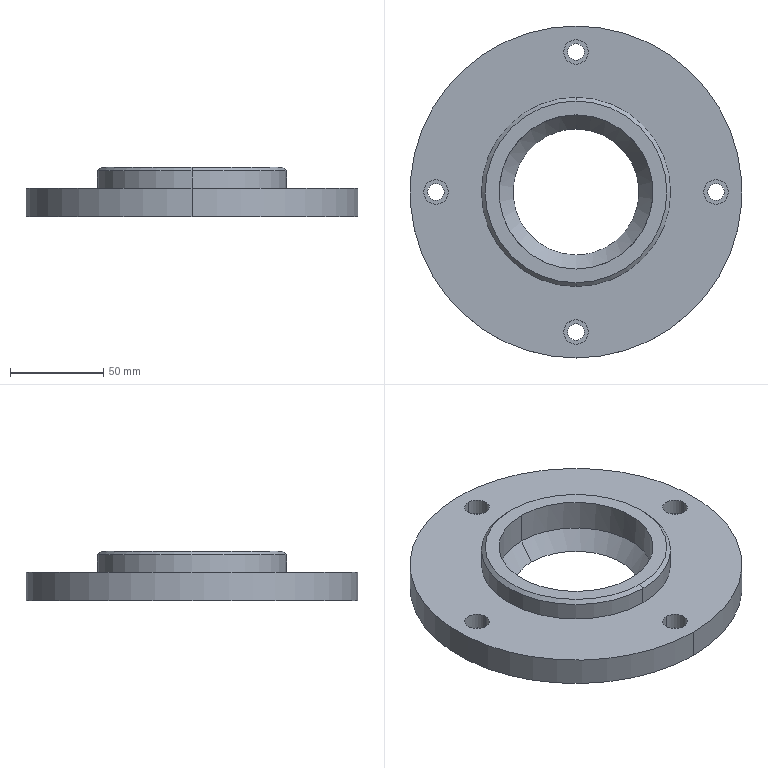Part | STEP file | 4-20.sldasm-Part-429 | 1 solid | 33 faces | box 177.8 x 177.8 x 26.75 mm | volume 331383 mm3 | cylinder 22 | plane 7 | spline 2 | cone 2 | commonest cylinder face diameters 8.931 x8 13.145 x8 82.56 x2 101.34 x2 177.8 x2
STEP:
#1=CARTESIAN_POINT('',(0.,81.572,313.382));
#2=VERTEX_POINT('',#1);
#3=CARTESIAN_POINT('',(0.,68.428,313.382));
#4=VERTEX_POINT('',#3);
#5=CARTESIAN_POINT('',(0.,75.,313.382));
#6=DIRECTION('',(0.,0.,1.));
#7=DIRECTION('',(0.,1.,0.));
#8=AXIS2_PLACEMENT_3D('',#5,#6,#7);
#9=CIRCLE('',#8,6.572);
#10=EDGE_CURVE('',#2,#4,#9,.T.);
#11=ORIENTED_EDGE('',*,*,#10,.F.);
#12=CARTESIAN_POINT('',(0.,81.572,322.275));
#13=VERTEX_POINT('',#12);
#14=CARTESIAN_POINT('',(0.,81.572,270.665));
#15=DIRECTION('',(0.,0.,1.));
#16=VECTOR('',#15,1000.);
#17=LINE('',#14,#16);
#18=EDGE_CURVE('',#2,#13,#17,.T.);
#19=ORIENTED_EDGE('',*,*,#18,.T.);
#20=CARTESIAN_POINT('',(0.,68.428,322.275));
#21=VERTEX_POINT('',#20);
#22=CARTESIAN_POINT('',(0.,75.,322.275));
#23=DIRECTION('',(0.,0.,-1.));
#24=DIRECTION('',(0.,-1.,0.));
#25=AXIS2_PLACEMENT_3D('',#22,#23,#24);
#26=CIRCLE('',#25,6.572);
#27=EDGE_CURVE('',#21,#13,#26,.T.);
#28=ORIENTED_EDGE('',*,*,#27,.F.);
#29=CARTESIAN_POINT('',(0.,68.428,270.665));
#30=DIRECTION('',(0.,0.,1.));
#31=VECTOR('',#30,1000.);
#32=LINE('',#29,#31);
#33=EDGE_CURVE('',#4,#21,#32,.T.);
#34=ORIENTED_EDGE('',*,*,#33,.F.);
#35=EDGE_LOOP('',(#11,#19,#28,#34));
#36=FACE_OUTER_BOUND('',#35,.T.);
#37=CARTESIAN_POINT('',(0.,75.,270.665));
#38=DIRECTION('',(0.,0.,1.));
#39=DIRECTION('',(0.,-1.,0.));
#40=AXIS2_PLACEMENT_3D('',#37,#38,#39);
#41=CYLINDRICAL_SURFACE('',#40,6.572);
#42=ADVANCED_FACE('',(#36),#41,.F.);
#43=CARTESIAN_POINT('',(-4.465,75.,313.382));
#44=VERTEX_POINT('',#43);
#45=CARTESIAN_POINT('',(4.465,75.,313.382));
#46=VERTEX_POINT('',#45);
#47=CARTESIAN_POINT('',(0.,75.,313.382));
#48=DIRECTION('',(0.,0.,-1.));
#49=DIRECTION('',(1.,0.,0.));
#50=AXIS2_PLACEMENT_3D('',#47,#48,#49);
#51=CIRCLE('',#50,4.465);
#52=EDGE_CURVE('',#44,#46,#51,.T.);
#53=ORIENTED_EDGE('',*,*,#52,.F.);
#54=CARTESIAN_POINT('',(-4.465,75.,306.955));
#55=VERTEX_POINT('',#54);
#56=CARTESIAN_POINT('',(-4.465,75.,313.382));
#57=DIRECTION('',(0.,0.,-1.));
#58=VECTOR('',#57,1000.);
#59=LINE('',#56,#58);
#60=EDGE_CURVE('',#44,#55,#59,.T.);
#61=ORIENTED_EDGE('',*,*,#60,.T.);
#62=CARTESIAN_POINT('',(4.465,75.,306.955));
#63=VERTEX_POINT('',#62);
#64=CARTESIAN_POINT('',(0.,75.,306.955));
#65=DIRECTION('',(0.,-0.000000019,1.));
#66=DIRECTION('',(0.,-1.,-0.000000019));
#67=AXIS2_PLACEMENT_3D('',#64,#65,#66);
#68=CIRCLE('',#67,4.465);
#69=EDGE_CURVE('',#63,#55,#68,.T.);
#70=ORIENTED_EDGE('',*,*,#69,.F.);
#71=CARTESIAN_POINT('',(4.465,75.,313.382));
#72=DIRECTION('',(0.,0.,-1.));
#73=VECTOR('',#72,1000.);
#74=LINE('',#71,#73);
#75=EDGE_CURVE('',#46,#63,#74,.T.);
#76=ORIENTED_EDGE('',*,*,#75,.F.);
#77=EDGE_LOOP('',(#53,#61,#70,#76));
#78=FACE_OUTER_BOUND('',#77,.T.);
#79=CARTESIAN_POINT('',(0.,75.,313.382));
#80=DIRECTION('',(0.,0.,-1.));
#81=DIRECTION('',(1.,0.,0.));
#82=AXIS2_PLACEMENT_3D('',#79,#80,#81);
#83=CYLINDRICAL_SURFACE('',#82,4.465);
#84=ADVANCED_FACE('',(#78),#83,.F.);
#85=CARTESIAN_POINT('',(81.572,0.,313.382));
#86=VERTEX_POINT('',#85);
#87=CARTESIAN_POINT('',(68.428,0.,313.382));
#88=VERTEX_POINT('',#87);
#89=CARTESIAN_POINT('',(75.,0.,313.382));
#90=DIRECTION('',(0.,0.,1.));
#91=DIRECTION('',(1.,0.,0.));
#92=AXIS2_PLACEMENT_3D('',#89,#90,#91);
#93=CIRCLE('',#92,6.572);
#94=EDGE_CURVE('',#86,#88,#93,.T.);
#95=ORIENTED_EDGE('',*,*,#94,.F.);
#96=CARTESIAN_POINT('',(81.572,0.,322.275));
#97=VERTEX_POINT('',#96);
#98=CARTESIAN_POINT('',(81.572,0.,270.665));
#99=DIRECTION('',(0.,0.,1.));
#100=VECTOR('',#99,1000.);
#101=LINE('',#98,#100);
#102=EDGE_CURVE('',#86,#97,#101,.T.);
#103=ORIENTED_EDGE('',*,*,#102,.T.);
#104=CARTESIAN_POINT('',(68.428,0.,322.275));
#105=VERTEX_POINT('',#104);
#106=CARTESIAN_POINT('',(75.,0.,322.275));
#107=DIRECTION('',(0.,0.,-1.));
#108=DIRECTION('',(-1.,0.,0.));
#109=AXIS2_PLACEMENT_3D('',#106,#107,#108);
#110=CIRCLE('',#109,6.572);
#111=EDGE_CURVE('',#105,#97,#110,.T.);
#112=ORIENTED_EDGE('',*,*,#111,.F.);
#113=CARTESIAN_POINT('',(68.428,0.,270.665));
#114=DIRECTION('',(0.,0.,1.));
#115=VECTOR('',#114,1000.);
#116=LINE('',#113,#115);
#117=EDGE_CURVE('',#88,#105,#116,.T.);
#118=ORIENTED_EDGE('',*,*,#117,.F.);
#119=EDGE_LOOP('',(#95,#103,#112,#118));
#120=FACE_OUTER_BOUND('',#119,.T.);
#121=CARTESIAN_POINT('',(75.,0.,270.665));
#122=DIRECTION('',(0.,0.,1.));
#123=DIRECTION('',(-1.,0.,0.));
#124=AXIS2_PLACEMENT_3D('',#121,#122,#123);
#125=CYLINDRICAL_SURFACE('',#124,6.572);
#126=ADVANCED_FACE('',(#120),#125,.F.);
#127=CARTESIAN_POINT('',(75.,4.465,313.382));
#128=VERTEX_POINT('',#127);
#129=CARTESIAN_POINT('',(75.,-4.465,313.382));
#130=VERTEX_POINT('',#129);
#131=CARTESIAN_POINT('',(75.,0.,313.382));
#132=DIRECTION('',(0.,0.,-1.));
#133=DIRECTION('',(0.,-1.,0.));
#134=AXIS2_PLACEMENT_3D('',#131,#132,#133);
#135=CIRCLE('',#134,4.465);
#136=EDGE_CURVE('',#128,#130,#135,.T.);
#137=ORIENTED_EDGE('',*,*,#136,.F.);
#138=CARTESIAN_POINT('',(75.,4.465,306.955));
#139=VERTEX_POINT('',#138);
#140=CARTESIAN_POINT('',(75.,4.465,313.382));
#141=DIRECTION('',(0.,0.,-1.));
#142=VECTOR('',#141,1000.);
#143=LINE('',#140,#142);
#144=EDGE_CURVE('',#128,#139,#143,.T.);
#145=ORIENTED_EDGE('',*,*,#144,.T.);
#146=CARTESIAN_POINT('',(75.,-4.465,306.955));
#147=VERTEX_POINT('',#146);
#148=CARTESIAN_POINT('',(75.,0.,306.955));
#149=DIRECTION('',(0.,-0.000000019,1.));
#150=DIRECTION('',(0.,-1.,-0.000000019));
#151=AXIS2_PLACEMENT_3D('',#148,#149,#150);
#152=CIRCLE('',#151,4.465);
#153=EDGE_CURVE('',#147,#139,#152,.T.);
#154=ORIENTED_EDGE('',*,*,#153,.F.);
#155=CARTESIAN_POINT('',(75.,-4.465,313.382));
#156=DIRECTION('',(0.,0.,-1.));
#157=VECTOR('',#156,1000.);
#158=LINE('',#155,#157);
#159=EDGE_CURVE('',#130,#147,#158,.T.);
#160=ORIENTED_EDGE('',*,*,#159,.F.);
#161=EDGE_LOOP('',(#137,#145,#154,#160));
#162=FACE_OUTER_BOUND('',#161,.T.);
#163=CARTESIAN_POINT('',(75.,0.,313.382));
#164=DIRECTION('',(0.,0.,-1.));
#165=DIRECTION('',(0.,-1.,0.));
#166=AXIS2_PLACEMENT_3D('',#163,#164,#165);
#167=CYLINDRICAL_SURFACE('',#166,4.465);
#168=ADVANCED_FACE('',(#162),#167,.F.);
#169=CARTESIAN_POINT('',(0.,-81.572,313.382));
#170=VERTEX_POINT('',#169);
#171=CARTESIAN_POINT('',(0.,-68.428,313.382));
#172=VERTEX_POINT('',#171);
#173=CARTESIAN_POINT('',(0.,-75.,313.382));
#174=DIRECTION('',(0.,0.,1.));
#175=DIRECTION('',(0.,-1.,0.));
#176=AXIS2_PLACEMENT_3D('',#173,#174,#175);
#177=CIRCLE('',#176,6.572);
#178=EDGE_CURVE('',#170,#172,#177,.T.);
#179=ORIENTED_EDGE('',*,*,#178,.F.);
#180=CARTESIAN_POINT('',(0.,-81.572,322.275));
#181=VERTEX_POINT('',#180);
#182=CARTESIAN_POINT('',(0.,-81.572,270.665));
#183=DIRECTION('',(0.,0.,1.));
#184=VECTOR('',#183,1000.);
#185=LINE('',#182,#184);
#186=EDGE_CURVE('',#170,#181,#185,.T.);
#187=ORIENTED_EDGE('',*,*,#186,.T.);
#188=CARTESIAN_POINT('',(0.,-68.428,322.275));
#189=VERTEX_POINT('',#188);
#190=CARTESIAN_POINT('',(0.,-75.,322.275));
#191=DIRECTION('',(0.,0.,-1.));
#192=DIRECTION('',(0.,1.,0.));
#193=AXIS2_PLACEMENT_3D('',#190,#191,#192);
#194=CIRCLE('',#193,6.572);
#195=EDGE_CURVE('',#189,#181,#194,.T.);
#196=ORIENTED_EDGE('',*,*,#195,.F.);
#197=CARTESIAN_POINT('',(0.,-68.428,270.665));
#198=DIRECTION('',(0.,0.,1.));
#199=VECTOR('',#198,1000.);
#200=LINE('',#197,#199);
#201=EDGE_CURVE('',#172,#189,#200,.T.);
#202=ORIENTED_EDGE('',*,*,#201,.F.);
#203=EDGE_LOOP('',(#179,#187,#196,#202));
#204=FACE_OUTER_BOUND('',#203,.T.);
#205=CARTESIAN_POINT('',(0.,-75.,270.665));
#206=DIRECTION('',(0.,0.,1.));
#207=DIRECTION('',(0.,1.,0.));
#208=AXIS2_PLACEMENT_3D('',#205,#206,#207);
#209=CYLINDRICAL_SURFACE('',#208,6.572);
#210=ADVANCED_FACE('',(#204),#209,.F.);
#211=CARTESIAN_POINT('',(4.465,-75.,313.382));
#212=VERTEX_POINT('',#211);
#213=CARTESIAN_POINT('',(-4.465,-75.,313.382));
#214=VERTEX_POINT('',#213);
#215=CARTESIAN_POINT('',(0.,-75.,313.382));
#216=DIRECTION('',(0.,0.,-1.));
#217=DIRECTION('',(-1.,0.,0.));
#218=AXIS2_PLACEMENT_3D('',#215,#216,#217);
#219=CIRCLE('',#218,4.465);
#220=EDGE_CURVE('',#212,#214,#219,.T.);
#221=ORIENTED_EDGE('',*,*,#220,.F.);
#222=CARTESIAN_POINT('',(4.465,-75.,306.955));
#223=VERTEX_POINT('',#222);
#224=CARTESIAN_POINT('',(4.465,-75.,313.382));
#225=DIRECTION('',(0.,0.,-1.));
#226=VECTOR('',#225,1000.);
#227=LINE('',#224,#226);
#228=EDGE_CURVE('',#212,#223,#227,.T.);
#229=ORIENTED_EDGE('',*,*,#228,.T.);
#230=CARTESIAN_POINT('',(-4.465,-75.,306.955));
#231=VERTEX_POINT('',#230);
#232=CARTESIAN_POINT('',(0.,-75.,306.955));
#233=DIRECTION('',(0.,-0.000000019,1.));
#234=DIRECTION('',(0.,-1.,-0.000000019));
#235=AXIS2_PLACEMENT_3D('',#232,#233,#234);
#236=CIRCLE('',#235,4.465);
#237=EDGE_CURVE('',#231,#223,#236,.T.);
#238=ORIENTED_EDGE('',*,*,#237,.F.);
#239=CARTESIAN_POINT('',(-4.465,-75.,313.382));
#240=DIRECTION('',(0.,0.,-1.));
#241=VECTOR('',#240,1000.);
#242=LINE('',#239,#241);
#243=EDGE_CURVE('',#214,#231,#242,.T.);
#244=ORIENTED_EDGE('',*,*,#243,.F.);
#245=EDGE_LOOP('',(#221,#229,#238,#244));
#246=FACE_OUTER_BOUND('',#245,.T.);
#247=CARTESIAN_POINT('',(0.,-75.,313.382));
#248=DIRECTION('',(0.,0.,-1.));
#249=DIRECTION('',(-1.,0.,0.));
#250=AXIS2_PLACEMENT_3D('',#247,#248,#249);
#251=CYLINDRICAL_SURFACE('',#250,4.465);
#252=ADVANCED_FACE('',(#246),#251,.F.);
#253=CARTESIAN_POINT('',(-81.572,0.,313.382));
#254=VERTEX_POINT('',#253);
#255=CARTESIAN_POINT('',(-68.428,0.,313.382));
#256=VERTEX_POINT('',#255);
#257=CARTESIAN_POINT('',(-75.,0.,313.382));
#258=DIRECTION('',(0.,0.,1.));
#259=DIRECTION('',(-1.,0.,0.));
#260=AXIS2_PLACEMENT_3D('',#257,#258,#259);
#261=CIRCLE('',#260,6.572);
#262=EDGE_CURVE('',#254,#256,#261,.T.);
#263=ORIENTED_EDGE('',*,*,#262,.F.);
#264=CARTESIAN_POINT('',(-81.572,0.,322.275));
#265=VERTEX_POINT('',#264);
#266=CARTESIAN_POINT('',(-81.572,0.,270.665));
#267=DIRECTION('',(0.,0.,1.));
#268=VECTOR('',#267,1000.);
#269=LINE('',#266,#268);
#270=EDGE_CURVE('',#254,#265,#269,.T.);
#271=ORIENTED_EDGE('',*,*,#270,.T.);
#272=CARTESIAN_POINT('',(-68.428,0.,322.275));
#273=VERTEX_POINT('',#272);
#274=CARTESIAN_POINT('',(-75.,0.,322.275));
#275=DIRECTION('',(0.,0.,-1.));
#276=DIRECTION('',(1.,0.,0.));
#277=AXIS2_PLACEMENT_3D('',#274,#275,#276);
#278=CIRCLE('',#277,6.572);
#279=EDGE_CURVE('',#273,#265,#278,.T.);
#280=ORIENTED_EDGE('',*,*,#279,.F.);
#281=CARTESIAN_POINT('',(-68.428,0.,270.665));
#282=DIRECTION('',(0.,0.,1.));
#283=VECTOR('',#282,1000.);
#284=LINE('',#281,#283);
#285=EDGE_CURVE('',#256,#273,#284,.T.);
#286=ORIENTED_EDGE('',*,*,#285,.F.);
#287=EDGE_LOOP('',(#263,#271,#280,#286));
#288=FACE_OUTER_BOUND('',#287,.T.);
#289=CARTESIAN_POINT('',(-75.,0.,270.665));
#290=DIRECTION('',(0.,0.,1.));
#291=DIRECTION('',(1.,0.,0.));
#292=AXIS2_PLACEMENT_3D('',#289,#290,#291);
#293=CYLINDRICAL_SURFACE('',#292,6.572);
#294=ADVANCED_FACE('',(#288),#293,.F.);
#295=CARTESIAN_POINT('',(-75.,-4.465,313.382));
#296=VERTEX_POINT('',#295);
#297=CARTESIAN_POINT('',(-75.,4.465,313.382));
#298=VERTEX_POINT('',#297);
#299=CARTESIAN_POINT('',(-75.,0.,313.382));
#300=DIRECTION('',(0.,0.,-1.));
#301=DIRECTION('',(0.,1.,0.));
#302=AXIS2_PLACEMENT_3D('',#299,#300,#301);
#303=CIRCLE('',#302,4.465);
#304=EDGE_CURVE('',#296,#298,#303,.T.);
#305=ORIENTED_EDGE('',*,*,#304,.F.);
#306=CARTESIAN_POINT('',(-75.,-4.465,306.955));
#307=VERTEX_POINT('',#306);
#308=CARTESIAN_POINT('',(-75.,-4.465,313.382));
#309=DIRECTION('',(0.,0.,-1.));
#310=VECTOR('',#309,1000.);
#311=LINE('',#308,#310);
#312=EDGE_CURVE('',#296,#307,#311,.T.);
#313=ORIENTED_EDGE('',*,*,#312,.T.);
#314=CARTESIAN_POINT('',(-75.,4.465,306.955));
#315=VERTEX_POINT('',#314);
#316=CARTESIAN_POINT('',(-75.,0.,306.955));
#317=DIRECTION('',(0.,-0.000000019,1.));
#318=DIRECTION('',(0.,-1.,-0.000000019));
#319=AXIS2_PLACEMENT_3D('',#316,#317,#318);
#320=CIRCLE('',#319,4.465);
#321=EDGE_CURVE('',#315,#307,#320,.T.);
#322=ORIENTED_EDGE('',*,*,#321,.F.);
#323=CARTESIAN_POINT('',(-75.,4.465,313.382));
#324=DIRECTION('',(0.,0.,-1.));
#325=VECTOR('',#324,1000.);
#326=LINE('',#323,#325);
#327=EDGE_CURVE('',#298,#315,#326,.T.);
#328=ORIENTED_EDGE('',*,*,#327,.F.);
#329=EDGE_LOOP('',(#305,#313,#322,#328));
#330=FACE_OUTER_BOUND('',#329,.T.);
#331=CARTESIAN_POINT('',(-75.,0.,313.382));
#332=DIRECTION('',(0.,0.,-1.));
#333=DIRECTION('',(0.,1.,0.));
#334=AXIS2_PLACEMENT_3D('',#331,#332,#333);
#335=CYLINDRICAL_SURFACE('',#334,4.465);
#336=ADVANCED_FACE('',(#330),#335,.F.);
#337=CARTESIAN_POINT('',(0.,-41.28,316.95));
#338=VERTEX_POINT('',#337);
#339=CARTESIAN_POINT('',(0.,41.28,316.95));
#340=VERTEX_POINT('',#339);
#341=CARTESIAN_POINT('',(0.,-41.28,316.95));
#342=CARTESIAN_POINT('',(14.595,-41.28,316.95));
#343=CARTESIAN_POINT('',(33.983,-33.983,316.95));
#344=CARTESIAN_POINT('',(41.28,-14.595,316.95));
#345=CARTESIAN_POINT('',(41.28,14.595,316.95));
#346=CARTESIAN_POINT('',(33.983,33.983,316.95));
#347=CARTESIAN_POINT('',(14.595,41.28,316.95));
#348=CARTESIAN_POINT('',(0.,41.28,316.95));
#349=(BOUNDED_CURVE()B_SPLINE_CURVE(4,(#341,#342,#343,#344,#345,#346,#347,#348),.UNSPECIFIED.,.F.,.F.)B_SPLINE_CURVE_WITH_KNOTS((5,3,5),(0.,0.25,0.5),.UNSPECIFIED.)CURVE()GEOMETRIC_REPRESENTATION_ITEM()RATIONAL_B_SPLINE_CURVE((1.017,1.017,0.9585,1.017,1.017,0.9585,1.017,1.017))REPRESENTATION_ITEM(''));
#350=EDGE_CURVE('',#338,#340,#349,.T.);
#351=ORIENTED_EDGE('',*,*,#350,.T.);
#352=CARTESIAN_POINT('',(0.,33.735,306.955));
#353=VERTEX_POINT('',#352);
#354=CARTESIAN_POINT('',(0.,41.28,316.95));
#355=CARTESIAN_POINT('',(0.,33.735,306.955));
#356=(BOUNDED_CURVE()B_SPLINE_CURVE(1,(#354,#355),.UNSPECIFIED.,.F.,.F.)B_SPLINE_CURVE_WITH_KNOTS((2,2),(0.,1.),.UNSPECIFIED.)CURVE()GEOMETRIC_REPRESENTATION_ITEM()RATIONAL_B_SPLINE_CURVE((1.017,1.017))REPRESENTATION_ITEM(''));
#357=EDGE_CURVE('',#340,#353,#356,.T.);
#358=ORIENTED_EDGE('',*,*,#357,.T.);
#359=CARTESIAN_POINT('',(0.,-33.735,306.955));
#360=VERTEX_POINT('',#359);
#361=CARTESIAN_POINT('',(0.,33.735,306.955));
#362=CARTESIAN_POINT('',(11.927,33.735,306.955));
#363=CARTESIAN_POINT('',(27.771,27.771,306.955));
#364=CARTESIAN_POINT('',(33.735,11.927,306.955));
#365=CARTESIAN_POINT('',(33.735,-11.927,306.955));
#366=CARTESIAN_POINT('',(27.771,-27.771,306.955));
#367=CARTESIAN_POINT('',(11.927,-33.735,306.955));
#368=CARTESIAN_POINT('',(0.,-33.735,306.955));
#369=(BOUNDED_CURVE()B_SPLINE_CURVE(4,(#361,#362,#363,#364,#365,#366,#367,#368),.UNSPECIFIED.,.F.,.F.)B_SPLINE_CURVE_WITH_KNOTS((5,3,5),(0.5,0.75,1.),.UNSPECIFIED.)CURVE()GEOMETRIC_REPRESENTATION_ITEM()RATIONAL_B_SPLINE_CURVE((1.017,1.017,0.9585,1.017,1.017,0.9585,1.017,1.017))REPRESENTATION_ITEM(''));
#370=EDGE_CURVE('',#353,#360,#369,.T.);
#371=ORIENTED_EDGE('',*,*,#370,.T.);
#372=CARTESIAN_POINT('',(0.,-41.28,316.95));
#373=CARTESIAN_POINT('',(0.,-33.735,306.955));
#374=(BOUNDED_CURVE()B_SPLINE_CURVE(1,(#372,#373),.UNSPECIFIED.,.F.,.T.)B_SPLINE_CURVE_WITH_KNOTS((2,2),(0.,1.),.UNSPECIFIED.)CURVE()GEOMETRIC_REPRESENTATION_ITEM()RATIONAL_B_SPLINE_CURVE((1.017,1.017))REPRESENTATION_ITEM(''));
#375=EDGE_CURVE('',#338,#360,#374,.T.);
#376=ORIENTED_EDGE('',*,*,#375,.F.);
#377=EDGE_LOOP('',(#351,#358,#371,#376));
#378=FACE_OUTER_BOUND('',#377,.T.);
#379=CARTESIAN_POINT('',(0.,-41.28,316.95));
#380=CARTESIAN_POINT('',(0.,-33.735,306.955));
#381=CARTESIAN_POINT('',(14.595,-41.28,316.95));
#382=CARTESIAN_POINT('',(11.927,-33.735,306.955));
#383=CARTESIAN_POINT('',(33.983,-33.983,316.95));
#384=CARTESIAN_POINT('',(27.771,-27.771,306.955));
#385=CARTESIAN_POINT('',(41.28,-14.595,316.95));
#386=CARTESIAN_POINT('',(33.735,-11.927,306.955));
#387=CARTESIAN_POINT('',(41.28,14.595,316.95));
#388=CARTESIAN_POINT('',(33.735,11.927,306.955));
#389=CARTESIAN_POINT('',(33.983,33.983,316.95));
#390=CARTESIAN_POINT('',(27.771,27.771,306.955));
#391=CARTESIAN_POINT('',(14.595,41.28,316.95));
#392=CARTESIAN_POINT('',(11.927,33.735,306.955));
#393=CARTESIAN_POINT('',(-14.595,41.28,316.95));
#394=CARTESIAN_POINT('',(-11.927,33.735,306.955));
#395=CARTESIAN_POINT('',(-33.983,33.983,316.95));
#396=CARTESIAN_POINT('',(-27.771,27.771,306.955));
#397=CARTESIAN_POINT('',(-41.28,14.595,316.95));
#398=CARTESIAN_POINT('',(-33.735,11.927,306.955));
#399=CARTESIAN_POINT('',(-41.28,-14.595,316.95));
#400=CARTESIAN_POINT('',(-33.735,-11.927,306.955));
#401=CARTESIAN_POINT('',(-33.983,-33.983,316.95));
#402=CARTESIAN_POINT('',(-27.771,-27.771,306.955));
#403=CARTESIAN_POINT('',(-14.595,-41.28,316.95));
#404=CARTESIAN_POINT('',(-11.927,-33.735,306.955));
#405=CARTESIAN_POINT('',(0.,-41.28,316.95));
#406=CARTESIAN_POINT('',(0.,-33.735,306.955));
#407=(BOUNDED_SURFACE()B_SPLINE_SURFACE(4,1,((#379,#380),(#381,#382),(#383,#384),(#385,#386),(#387,#388),(#389,#390),(#391,#392),(#393,#394),(#395,#396),(#397,#398),(#399,#400),(#401,#402),(#403,#404),(#405,#406)),.UNSPECIFIED.,.T.,.F.,.F.)B_SPLINE_SURFACE_WITH_KNOTS((5,3,3,3,5),(2,2),(0.,0.25,0.5,0.75,1.),(0.,1.),.UNSPECIFIED.)GEOMETRIC_REPRESENTATION_ITEM()RATIONAL_B_SPLINE_SURFACE(((1.017,1.017),(1.017,1.017),(0.9585,0.9585),(1.017,1.017),(1.017,1.017),(0.9585,0.9585),(1.017,1.017),(1.017,1.017),(0.9585,0.9585),(1.017,1.017),(1.017,1.017),(0.9585,0.9585),(1.017,1.017),(1.017,1.017)))REPRESENTATION_ITEM('')SURFACE());
#408=ADVANCED_FACE('',(#378),#407,.T.);
#409=CARTESIAN_POINT('',(0.,41.28,316.95));
#410=CARTESIAN_POINT('',(-14.595,41.28,316.95));
#411=CARTESIAN_POINT('',(-33.983,33.983,316.95));
#412=CARTESIAN_POINT('',(-41.28,14.595,316.95));
#413=CARTESIAN_POINT('',(-41.28,-14.595,316.95));
#414=CARTESIAN_POINT('',(-33.983,-33.983,316.95));
#415=CARTESIAN_POINT('',(-14.595,-41.28,316.95));
#416=CARTESIAN_POINT('',(0.,-41.28,316.95));
#417=(BOUNDED_CURVE()B_SPLINE_CURVE(4,(#409,#410,#411,#412,#413,#414,#415,#416),.UNSPECIFIED.,.F.,.F.)B_SPLINE_CURVE_WITH_KNOTS((5,3,5),(0.5,0.75,1.),.UNSPECIFIED.)CURVE()GEOMETRIC_REPRESENTATION_ITEM()RATIONAL_B_SPLINE_CURVE((1.017,1.017,0.9585,1.017,1.017,0.9585,1.017,1.017))REPRESENTATION_ITEM(''));
#418=EDGE_CURVE('',#340,#338,#417,.T.);
#419=ORIENTED_EDGE('',*,*,#418,.F.);
#420=CARTESIAN_POINT('',(0.,41.28,333.705));
#421=VERTEX_POINT('',#420);
#422=CARTESIAN_POINT('',(0.,41.28,333.973));
#423=DIRECTION('',(0.,-0.000000019,1.));
#424=VECTOR('',#423,1000.);
#425=LINE('',#422,#424);
#426=EDGE_CURVE('',#340,#421,#425,.T.);
#427=ORIENTED_EDGE('',*,*,#426,.T.);
#428=CARTESIAN_POINT('',(0.,-41.28,333.705));
#429=VERTEX_POINT('',#428);
#430=CARTESIAN_POINT('',(0.,-0.000003929,333.705));
#431=DIRECTION('',(0.,-0.000000019,1.));
#432=DIRECTION('',(0.,-1.,-0.000000019));
#433=AXIS2_PLACEMENT_3D('',#430,#431,#432);
#434=CIRCLE('',#433,41.28);
#435=EDGE_CURVE('',#421,#429,#434,.T.);
#436=ORIENTED_EDGE('',*,*,#435,.T.);
#437=CARTESIAN_POINT('',(0.,-41.28,333.973));
#438=DIRECTION('',(0.,-0.000000019,1.));
#439=VECTOR('',#438,1000.);
#440=LINE('',#437,#439);
#441=EDGE_CURVE('',#338,#429,#440,.T.);
#442=ORIENTED_EDGE('',*,*,#441,.F.);
#443=EDGE_LOOP('',(#419,#427,#436,#442));
#444=FACE_OUTER_BOUND('',#443,.T.);
#445=CARTESIAN_POINT('',(0.,-0.000003934,333.973));
#446=DIRECTION('',(0.,-0.000000019,1.));
#447=DIRECTION('',(0.,-1.,-0.000000019));
#448=AXIS2_PLACEMENT_3D('',#445,#446,#447);
#449=CYLINDRICAL_SURFACE('',#448,41.28);
#450=ADVANCED_FACE('',(#444),#449,.F.);
#451=CARTESIAN_POINT('',(0.,-50.67,322.275));
#452=VERTEX_POINT('',#451);
#453=CARTESIAN_POINT('',(0.,50.67,322.275));
#454=VERTEX_POINT('',#453);
#455=CARTESIAN_POINT('',(0.,-0.000003901,322.275));
#456=DIRECTION('',(0.,-0.000000019,1.));
#457=DIRECTION('',(0.,-1.,-0.000000019));
#458=AXIS2_PLACEMENT_3D('',#455,#456,#457);
#459=CIRCLE('',#458,50.67);
#460=EDGE_CURVE('',#452,#454,#459,.T.);
#461=ORIENTED_EDGE('',*,*,#460,.T.);
#462=CARTESIAN_POINT('',(0.,50.67,331.705));
#463=VERTEX_POINT('',#462);
#464=CARTESIAN_POINT('',(0.,50.67,323.978));
#465=DIRECTION('',(0.,-0.000000019,1.));
#466=VECTOR('',#465,1000.);
#467=LINE('',#464,#466);
#468=EDGE_CURVE('',#454,#463,#467,.T.);
#469=ORIENTED_EDGE('',*,*,#468,.T.);
#470=CARTESIAN_POINT('',(0.,-50.67,331.705));
#471=VERTEX_POINT('',#470);
#472=CARTESIAN_POINT('',(0.,-0.000004083,331.705));
#473=DIRECTION('',(0.,-0.000000019,1.));
#474=DIRECTION('',(0.,-1.,-0.000000019));
#475=AXIS2_PLACEMENT_3D('',#472,#473,#474);
#476=CIRCLE('',#475,50.67);
#477=EDGE_CURVE('',#471,#463,#476,.T.);
#478=ORIENTED_EDGE('',*,*,#477,.F.);
#479=CARTESIAN_POINT('',(0.,-50.67,323.978));
#480=DIRECTION('',(0.,-0.000000019,1.));
#481=VECTOR('',#480,1000.);
#482=LINE('',#479,#481);
#483=EDGE_CURVE('',#452,#471,#482,.T.);
#484=ORIENTED_EDGE('',*,*,#483,.F.);
#485=EDGE_LOOP('',(#461,#469,#478,#484));
#486=FACE_OUTER_BOUND('',#485,.T.);
#487=CARTESIAN_POINT('',(0.,-0.000003934,323.978));
#488=DIRECTION('',(0.,-0.000000019,1.));
#489=DIRECTION('',(0.,-1.,-0.000000019));
#490=AXIS2_PLACEMENT_3D('',#487,#488,#489);
#491=CYLINDRICAL_SURFACE('',#490,50.67);
#492=ADVANCED_FACE('',(#486),#491,.T.);
#493=CARTESIAN_POINT('',(0.,-48.67,333.705));
#494=VERTEX_POINT('',#493);
#495=CARTESIAN_POINT('',(0.,48.67,333.705));
#496=VERTEX_POINT('',#495);
#497=CARTESIAN_POINT('',(0.,-0.000004121,333.705));
#498=DIRECTION('',(0.,-0.000000019,1.));
#499=DIRECTION('',(0.,-1.,-0.000000019));
#500=AXIS2_PLACEMENT_3D('',#497,#498,#499);
#501=CIRCLE('',#500,48.67);
#502=EDGE_CURVE('',#494,#496,#501,.T.);
#503=ORIENTED_EDGE('',*,*,#502,.F.);
#504=CARTESIAN_POINT('',(0.,-50.67,331.705));
#505=DIRECTION('',(0.,-0.7071,-0.7071));
#506=VECTOR('',#505,1000.);
#507=LINE('',#504,#506);
#508=EDGE_CURVE('',#494,#471,#507,.T.);
#509=ORIENTED_EDGE('',*,*,#508,.T.);
#510=ORIENTED_EDGE('',*,*,#477,.T.);
#511=CARTESIAN_POINT('',(0.,50.67,331.705));
#512=DIRECTION('',(0.,0.7071,-0.7071));
#513=VECTOR('',#512,1000.);
#514=LINE('',#511,#513);
#515=EDGE_CURVE('',#496,#463,#514,.T.);
#516=ORIENTED_EDGE('',*,*,#515,.F.);
#517=EDGE_LOOP('',(#503,#509,#510,#516));
#518=FACE_OUTER_BOUND('',#517,.T.);
#519=CARTESIAN_POINT('',(0.,-0.000004083,331.705));
#520=DIRECTION('',(0.,0.000000019,-1.));
#521=DIRECTION('',(0.,1.,0.000000019));
#522=AXIS2_PLACEMENT_3D('',#519,#520,#521);
#523=CONICAL_SURFACE('',#522,50.67,0.7854);
#524=ADVANCED_FACE('',(#518),#523,.T.);
#525=CARTESIAN_POINT('',(0.,-88.9,306.955));
#526=VERTEX_POINT('',#525);
#527=CARTESIAN_POINT('',(0.,88.9,306.955));
#528=VERTEX_POINT('',#527);
#529=CARTESIAN_POINT('',(0.,-0.000003607,306.955));
#530=DIRECTION('',(0.,-0.000000019,1.));
#531=DIRECTION('',(0.,-1.,-0.000000019));
#532=AXIS2_PLACEMENT_3D('',#529,#530,#531);
#533=CIRCLE('',#532,88.9);
#534=EDGE_CURVE('',#526,#528,#533,.T.);
#535=ORIENTED_EDGE('',*,*,#534,.T.);
#536=CARTESIAN_POINT('',(0.,88.9,322.275));
#537=VERTEX_POINT('',#536);
#538=CARTESIAN_POINT('',(0.,88.9,323.978));
#539=DIRECTION('',(0.,-0.000000019,1.));
#540=VECTOR('',#539,1000.);
#541=LINE('',#538,#540);
#542=EDGE_CURVE('',#528,#537,#541,.T.);
#543=ORIENTED_EDGE('',*,*,#542,.T.);
#544=CARTESIAN_POINT('',(0.,-88.9,322.275));
#545=VERTEX_POINT('',#544);
#546=CARTESIAN_POINT('',(0.,-0.000003901,322.275));
#547=DIRECTION('',(0.,-0.000000019,1.));
#548=DIRECTION('',(0.,-1.,-0.000000019));
#549=AXIS2_PLACEMENT_3D('',#546,#547,#548);
#550=CIRCLE('',#549,88.9);
#551=EDGE_CURVE('',#545,#537,#550,.T.);
#552=ORIENTED_EDGE('',*,*,#551,.F.);
#553=CARTESIAN_POINT('',(0.,-88.9,323.978));
#554=DIRECTION('',(0.,-0.000000019,1.));
#555=VECTOR('',#554,1000.);
#556=LINE('',#553,#555);
#557=EDGE_CURVE('',#526,#545,#556,.T.);
#558=ORIENTED_EDGE('',*,*,#557,.F.);
#559=EDGE_LOOP('',(#535,#543,#552,#558));
#560=FACE_OUTER_BOUND('',#559,.T.);
#561=CARTESIAN_POINT('',(0.,-0.000003934,323.978));
#562=DIRECTION('',(0.,-0.000000019,1.));
#563=DIRECTION('',(0.,-1.,-0.000000019));
#564=AXIS2_PLACEMENT_3D('',#561,#562,#563);
#565=CYLINDRICAL_SURFACE('',#564,88.9);
#566=ADVANCED_FACE('',(#560),#565,.T.);
#567=ORIENTED_EDGE('',*,*,#111,.T.);
#568=CARTESIAN_POINT('',(75.,0.,322.275));
#569=DIRECTION('',(0.,0.,-1.));
#570=DIRECTION('',(-1.,0.,0.));
#571=AXIS2_PLACEMENT_3D('',#568,#569,#570);
#572=CIRCLE('',#571,6.572);
#573=EDGE_CURVE('',#97,#105,#572,.T.);
#574=ORIENTED_EDGE('',*,*,#573,.T.);
#575=EDGE_LOOP('',(#567,#574));
#576=FACE_BOUND('',#575,.T.);
#577=ORIENTED_EDGE('',*,*,#279,.T.);
#578=CARTESIAN_POINT('',(-75.,0.,322.275));
#579=DIRECTION('',(0.,0.,-1.));
#580=DIRECTION('',(1.,0.,0.));
#581=AXIS2_PLACEMENT_3D('',#578,#579,#580);
#582=CIRCLE('',#581,6.572);
#583=EDGE_CURVE('',#265,#273,#582,.T.);
#584=ORIENTED_EDGE('',*,*,#583,.T.);
#585=EDGE_LOOP('',(#577,#584));
#586=FACE_BOUND('',#585,.T.);
#587=ORIENTED_EDGE('',*,*,#460,.F.);
#588=CARTESIAN_POINT('',(0.,-0.000003901,322.275));
#589=DIRECTION('',(0.,-0.000000019,1.));
#590=DIRECTION('',(0.,-1.,-0.000000019));
#591=AXIS2_PLACEMENT_3D('',#588,#589,#590);
#592=CIRCLE('',#591,50.67);
#593=EDGE_CURVE('',#454,#452,#592,.T.);
#594=ORIENTED_EDGE('',*,*,#593,.F.);
#595=EDGE_LOOP('',(#587,#594));
#596=FACE_BOUND('',#595,.T.);
#597=ORIENTED_EDGE('',*,*,#551,.T.);
#598=CARTESIAN_POINT('',(0.,-0.000003901,322.275));
#599=DIRECTION('',(0.,-0.000000019,1.));
#600=DIRECTION('',(0.,-1.,-0.000000019));
#601=AXIS2_PLACEMENT_3D('',#598,#599,#600);
#602=CIRCLE('',#601,88.9);
#603=EDGE_CURVE('',#537,#545,#602,.T.);
#604=ORIENTED_EDGE('',*,*,#603,.T.);
#605=EDGE_LOOP('',(#597,#604));
#606=FACE_OUTER_BOUND('',#605,.T.);
#607=ORIENTED_EDGE('',*,*,#195,.T.);
#608=CARTESIAN_POINT('',(0.,-75.,322.275));
#609=DIRECTION('',(0.,0.,-1.));
#610=DIRECTION('',(0.,1.,0.));
#611=AXIS2_PLACEMENT_3D('',#608,#609,#610);
#612=CIRCLE('',#611,6.572);
#613=EDGE_CURVE('',#181,#189,#612,.T.);
#614=ORIENTED_EDGE('',*,*,#613,.T.);
#615=EDGE_LOOP('',(#607,#614));
#616=FACE_BOUND('',#615,.T.);
#617=ORIENTED_EDGE('',*,*,#27,.T.);
#618=CARTESIAN_POINT('',(0.,75.,322.275));
#619=DIRECTION('',(0.,0.,-1.));
#620=DIRECTION('',(0.,-1.,0.));
#621=AXIS2_PLACEMENT_3D('',#618,#619,#620);
#622=CIRCLE('',#621,6.572);
#623=EDGE_CURVE('',#13,#21,#622,.T.);
#624=ORIENTED_EDGE('',*,*,#623,.T.);
#625=EDGE_LOOP('',(#617,#624));
#626=FACE_BOUND('',#625,.T.);
#627=CARTESIAN_POINT('',(0.,-0.000003901,322.275));
#628=DIRECTION('',(0.,-0.000000019,1.));
#629=DIRECTION('',(0.,-1.,-0.000000019));
#630=AXIS2_PLACEMENT_3D('',#627,#628,#629);
#631=PLANE('',#630);
#632=ADVANCED_FACE('',(#576,#586,#596,#606,#616,#626),#631,.T.);
#633=ORIENTED_EDGE('',*,*,#69,.T.);
#634=CARTESIAN_POINT('',(0.,75.,306.955));
#635=DIRECTION('',(0.,-0.000000019,1.));
#636=DIRECTION('',(0.,-1.,-0.000000019));
#637=AXIS2_PLACEMENT_3D('',#634,#635,#636);
#638=CIRCLE('',#637,4.465);
#639=EDGE_CURVE('',#55,#63,#638,.T.);
#640=ORIENTED_EDGE('',*,*,#639,.T.);
#641=EDGE_LOOP('',(#633,#640));
#642=FACE_BOUND('',#641,.T.);
#643=ORIENTED_EDGE('',*,*,#153,.T.);
#644=CARTESIAN_POINT('',(75.,0.,306.955));
#645=DIRECTION('',(0.,-0.000000019,1.));
#646=DIRECTION('',(0.,-1.,-0.000000019));
#647=AXIS2_PLACEMENT_3D('',#644,#645,#646);
#648=CIRCLE('',#647,4.465);
#649=EDGE_CURVE('',#139,#147,#648,.T.);
#650=ORIENTED_EDGE('',*,*,#649,.T.);
#651=EDGE_LOOP('',(#643,#650));
#652=FACE_BOUND('',#651,.T.);
#653=ORIENTED_EDGE('',*,*,#237,.T.);
#654=CARTESIAN_POINT('',(0.,-75.,306.955));
#655=DIRECTION('',(0.,-0.000000019,1.));
#656=DIRECTION('',(0.,-1.,-0.000000019));
#657=AXIS2_PLACEMENT_3D('',#654,#655,#656);
#658=CIRCLE('',#657,4.465);
#659=EDGE_CURVE('',#223,#231,#658,.T.);
#660=ORIENTED_EDGE('',*,*,#659,.T.);
#661=EDGE_LOOP('',(#653,#660));
#662=FACE_BOUND('',#661,.T.);
#663=ORIENTED_EDGE('',*,*,#321,.T.);
#664=CARTESIAN_POINT('',(-75.,0.,306.955));
#665=DIRECTION('',(0.,-0.000000019,1.));
#666=DIRECTION('',(0.,-1.,-0.000000019));
#667=AXIS2_PLACEMENT_3D('',#664,#665,#666);
#668=CIRCLE('',#667,4.465);
#669=EDGE_CURVE('',#307,#315,#668,.T.);
#670=ORIENTED_EDGE('',*,*,#669,.T.);
#671=EDGE_LOOP('',(#663,#670));
#672=FACE_BOUND('',#671,.T.);
#673=ORIENTED_EDGE('',*,*,#534,.F.);
#674=CARTESIAN_POINT('',(0.,-0.000003607,306.955));
#675=DIRECTION('',(0.,-0.000000019,1.));
#676=DIRECTION('',(0.,-1.,-0.000000019));
#677=AXIS2_PLACEMENT_3D('',#674,#675,#676);
#678=CIRCLE('',#677,88.9);
#679=EDGE_CURVE('',#528,#526,#678,.T.);
#680=ORIENTED_EDGE('',*,*,#679,.F.);
#681=EDGE_LOOP('',(#673,#680));
#682=FACE_OUTER_BOUND('',#681,.T.);
#683=CARTESIAN_POINT('',(0.,-33.735,306.955));
#684=CARTESIAN_POINT('',(-11.927,-33.735,306.955));
#685=CARTESIAN_POINT('',(-27.771,-27.771,306.955));
#686=CARTESIAN_POINT('',(-33.735,-11.927,306.955));
#687=CARTESIAN_POINT('',(-33.735,11.927,306.955));
#688=CARTESIAN_POINT('',(-27.771,27.771,306.955));
#689=CARTESIAN_POINT('',(-11.927,33.735,306.955));
#690=CARTESIAN_POINT('',(0.,33.735,306.955));
#691=(BOUNDED_CURVE()B_SPLINE_CURVE(4,(#683,#684,#685,#686,#687,#688,#689,#690),.UNSPECIFIED.,.F.,.F.)B_SPLINE_CURVE_WITH_KNOTS((5,3,5),(0.,0.25,0.5),.UNSPECIFIED.)CURVE()GEOMETRIC_REPRESENTATION_ITEM()RATIONAL_B_SPLINE_CURVE((1.017,1.017,0.9585,1.017,1.017,0.9585,1.017,1.017))REPRESENTATION_ITEM(''));
#692=EDGE_CURVE('',#360,#353,#691,.T.);
#693=ORIENTED_EDGE('',*,*,#692,.F.);
#694=ORIENTED_EDGE('',*,*,#370,.F.);
#695=EDGE_LOOP('',(#693,#694));
#696=FACE_BOUND('',#695,.T.);
#697=CARTESIAN_POINT('',(0.,-0.000003607,306.955));
#698=DIRECTION('',(0.,-0.000000019,1.));
#699=DIRECTION('',(0.,-1.,-0.000000019));
#700=AXIS2_PLACEMENT_3D('',#697,#698,#699);
#701=PLANE('',#700);
#702=ADVANCED_FACE('',(#642,#652,#662,#672,#682,#696),#701,.F.);
#703=ORIENTED_EDGE('',*,*,#542,.F.);
#704=ORIENTED_EDGE('',*,*,#679,.T.);
#705=ORIENTED_EDGE('',*,*,#557,.T.);
#706=ORIENTED_EDGE('',*,*,#603,.F.);
#707=EDGE_LOOP('',(#703,#704,#705,#706));
#708=FACE_OUTER_BOUND('',#707,.T.);
#709=CARTESIAN_POINT('',(0.,-0.000003934,323.978));
#710=DIRECTION('',(0.,-0.000000019,1.));
#711=DIRECTION('',(0.,-1.,-0.000000019));
#712=AXIS2_PLACEMENT_3D('',#709,#710,#711);
#713=CYLINDRICAL_SURFACE('',#712,88.9);
#714=ADVANCED_FACE('',(#708),#713,.T.);
#715=ORIENTED_EDGE('',*,*,#468,.F.);
#716=ORIENTED_EDGE('',*,*,#593,.T.);
#717=ORIENTED_EDGE('',*,*,#483,.T.);
#718=CARTESIAN_POINT('',(0.,-0.000004083,331.705));
#719=DIRECTION('',(0.,-0.000000019,1.));
#720=DIRECTION('',(0.,-1.,-0.000000019));
#721=AXIS2_PLACEMENT_3D('',#718,#719,#720);
#722=CIRCLE('',#721,50.67);
#723=EDGE_CURVE('',#463,#471,#722,.T.);
#724=ORIENTED_EDGE('',*,*,#723,.F.);
#725=EDGE_LOOP('',(#715,#716,#717,#724));
#726=FACE_OUTER_BOUND('',#725,.T.);
#727=CARTESIAN_POINT('',(0.,-0.000003934,323.978));
#728=DIRECTION('',(0.,-0.000000019,1.));
#729=DIRECTION('',(0.,-1.,-0.000000019));
#730=AXIS2_PLACEMENT_3D('',#727,#728,#729);
#731=CYLINDRICAL_SURFACE('',#730,50.67);
#732=ADVANCED_FACE('',(#726),#731,.T.);
#733=ORIENTED_EDGE('',*,*,#508,.F.);
#734=CARTESIAN_POINT('',(0.,-0.000004121,333.705));
#735=DIRECTION('',(0.,-0.000000019,1.));
#736=DIRECTION('',(0.,-1.,-0.000000019));
#737=AXIS2_PLACEMENT_3D('',#734,#735,#736);
#738=CIRCLE('',#737,48.67);
#739=EDGE_CURVE('',#496,#494,#738,.T.);
#740=ORIENTED_EDGE('',*,*,#739,.F.);
#741=ORIENTED_EDGE('',*,*,#515,.T.);
#742=ORIENTED_EDGE('',*,*,#723,.T.);
#743=EDGE_LOOP('',(#733,#740,#741,#742));
#744=FACE_OUTER_BOUND('',#743,.T.);
#745=CARTESIAN_POINT('',(0.,-0.000004083,331.705));
#746=DIRECTION('',(0.,0.000000019,-1.));
#747=DIRECTION('',(0.,1.,0.000000019));
#748=AXIS2_PLACEMENT_3D('',#745,#746,#747);
#749=CONICAL_SURFACE('',#748,50.67,0.7854);
#750=ADVANCED_FACE('',(#744),#749,.T.);
#751=CARTESIAN_POINT('',(0.,-0.000003929,333.705));
#752=DIRECTION('',(0.,-0.000000019,1.));
#753=DIRECTION('',(0.,-1.,-0.000000019));
#754=AXIS2_PLACEMENT_3D('',#751,#752,#753);
#755=CIRCLE('',#754,41.28);
#756=EDGE_CURVE('',#429,#421,#755,.T.);
#757=ORIENTED_EDGE('',*,*,#756,.F.);
#758=ORIENTED_EDGE('',*,*,#435,.F.);
#759=EDGE_LOOP('',(#757,#758));
#760=FACE_BOUND('',#759,.T.);
#761=ORIENTED_EDGE('',*,*,#739,.T.);
#762=ORIENTED_EDGE('',*,*,#502,.T.);
#763=EDGE_LOOP('',(#761,#762));
#764=FACE_OUTER_BOUND('',#763,.T.);
#765=CARTESIAN_POINT('',(0.,-0.000004121,333.705));
#766=DIRECTION('',(0.,-0.000000019,1.));
#767=DIRECTION('',(0.,-1.,-0.000000019));
#768=AXIS2_PLACEMENT_3D('',#765,#766,#767);
#769=PLANE('',#768);
#770=ADVANCED_FACE('',(#760,#764),#769,.T.);
#771=ORIENTED_EDGE('',*,*,#426,.F.);
#772=ORIENTED_EDGE('',*,*,#350,.F.);
#773=ORIENTED_EDGE('',*,*,#441,.T.);
#774=ORIENTED_EDGE('',*,*,#756,.T.);
#775=EDGE_LOOP('',(#771,#772,#773,#774));
#776=FACE_OUTER_BOUND('',#775,.T.);
#777=CARTESIAN_POINT('',(0.,-0.000003934,333.973));
#778=DIRECTION('',(0.,-0.000000019,1.));
#779=DIRECTION('',(0.,-1.,-0.000000019));
#780=AXIS2_PLACEMENT_3D('',#777,#778,#779);
#781=CYLINDRICAL_SURFACE('',#780,41.28);
#782=ADVANCED_FACE('',(#776),#781,.F.);
#783=ORIENTED_EDGE('',*,*,#357,.F.);
#784=ORIENTED_EDGE('',*,*,#418,.T.);
#785=ORIENTED_EDGE('',*,*,#375,.T.);
#786=ORIENTED_EDGE('',*,*,#692,.T.);
#787=EDGE_LOOP('',(#783,#784,#785,#786));
#788=FACE_OUTER_BOUND('',#787,.T.);
#789=CARTESIAN_POINT('',(0.,-41.28,316.95));
#790=CARTESIAN_POINT('',(0.,-33.735,306.955));
#791=CARTESIAN_POINT('',(14.595,-41.28,316.95));
#792=CARTESIAN_POINT('',(11.927,-33.735,306.955));
#793=CARTESIAN_POINT('',(33.983,-33.983,316.95));
#794=CARTESIAN_POINT('',(27.771,-27.771,306.955));
#795=CARTESIAN_POINT('',(41.28,-14.595,316.95));
#796=CARTESIAN_POINT('',(33.735,-11.927,306.955));
#797=CARTESIAN_POINT('',(41.28,14.595,316.95));
#798=CARTESIAN_POINT('',(33.735,11.927,306.955));
#799=CARTESIAN_POINT('',(33.983,33.983,316.95));
#800=CARTESIAN_POINT('',(27.771,27.771,306.955));
#801=CARTESIAN_POINT('',(14.595,41.28,316.95));
#802=CARTESIAN_POINT('',(11.927,33.735,306.955));
#803=CARTESIAN_POINT('',(-14.595,41.28,316.95));
#804=CARTESIAN_POINT('',(-11.927,33.735,306.955));
#805=CARTESIAN_POINT('',(-33.983,33.983,316.95));
#806=CARTESIAN_POINT('',(-27.771,27.771,306.955));
#807=CARTESIAN_POINT('',(-41.28,14.595,316.95));
#808=CARTESIAN_POINT('',(-33.735,11.927,306.955));
#809=CARTESIAN_POINT('',(-41.28,-14.595,316.95));
#810=CARTESIAN_POINT('',(-33.735,-11.927,306.955));
#811=CARTESIAN_POINT('',(-33.983,-33.983,316.95));
#812=CARTESIAN_POINT('',(-27.771,-27.771,306.955));
#813=CARTESIAN_POINT('',(-14.595,-41.28,316.95));
#814=CARTESIAN_POINT('',(-11.927,-33.735,306.955));
#815=CARTESIAN_POINT('',(0.,-41.28,316.95));
#816=CARTESIAN_POINT('',(0.,-33.735,306.955));
#817=(BOUNDED_SURFACE()B_SPLINE_SURFACE(4,1,((#789,#790),(#791,#792),(#793,#794),(#795,#796),(#797,#798),(#799,#800),(#801,#802),(#803,#804),(#805,#806),(#807,#808),(#809,#810),(#811,#812),(#813,#814),(#815,#816)),.UNSPECIFIED.,.T.,.F.,.F.)B_SPLINE_SURFACE_WITH_KNOTS((5,3,3,3,5),(2,2),(0.,0.25,0.5,0.75,1.),(0.,1.),.UNSPECIFIED.)GEOMETRIC_REPRESENTATION_ITEM()RATIONAL_B_SPLINE_SURFACE(((1.017,1.017),(1.017,1.017),(0.9585,0.9585),(1.017,1.017),(1.017,1.017),(0.9585,0.9585),(1.017,1.017),(1.017,1.017),(0.9585,0.9585),(1.017,1.017),(1.017,1.017),(0.9585,0.9585),(1.017,1.017),(1.017,1.017)))REPRESENTATION_ITEM('')SURFACE());
#818=ADVANCED_FACE('',(#788),#817,.T.);
#819=ORIENTED_EDGE('',*,*,#312,.F.);
#820=CARTESIAN_POINT('',(-75.,0.,313.382));
#821=DIRECTION('',(0.,0.,-1.));
#822=DIRECTION('',(0.,1.,0.));
#823=AXIS2_PLACEMENT_3D('',#820,#821,#822);
#824=CIRCLE('',#823,4.465);
#825=EDGE_CURVE('',#298,#296,#824,.T.);
#826=ORIENTED_EDGE('',*,*,#825,.F.);
#827=ORIENTED_EDGE('',*,*,#327,.T.);
#828=ORIENTED_EDGE('',*,*,#669,.F.);
#829=EDGE_LOOP('',(#819,#826,#827,#828));
#830=FACE_OUTER_BOUND('',#829,.T.);
#831=CARTESIAN_POINT('',(-75.,0.,313.382));
#832=DIRECTION('',(0.,0.,-1.));
#833=DIRECTION('',(0.,1.,0.));
#834=AXIS2_PLACEMENT_3D('',#831,#832,#833);
#835=CYLINDRICAL_SURFACE('',#834,4.465);
#836=ADVANCED_FACE('',(#830),#835,.F.);
#837=ORIENTED_EDGE('',*,*,#270,.F.);
#838=CARTESIAN_POINT('',(-75.,0.,313.382));
#839=DIRECTION('',(0.,0.,1.));
#840=DIRECTION('',(-1.,0.,0.));
#841=AXIS2_PLACEMENT_3D('',#838,#839,#840);
#842=CIRCLE('',#841,6.572);
#843=EDGE_CURVE('',#256,#254,#842,.T.);
#844=ORIENTED_EDGE('',*,*,#843,.F.);
#845=ORIENTED_EDGE('',*,*,#285,.T.);
#846=ORIENTED_EDGE('',*,*,#583,.F.);
#847=EDGE_LOOP('',(#837,#844,#845,#846));
#848=FACE_OUTER_BOUND('',#847,.T.);
#849=CARTESIAN_POINT('',(-75.,0.,270.665));
#850=DIRECTION('',(0.,0.,1.));
#851=DIRECTION('',(1.,0.,0.));
#852=AXIS2_PLACEMENT_3D('',#849,#850,#851);
#853=CYLINDRICAL_SURFACE('',#852,6.572);
#854=ADVANCED_FACE('',(#848),#853,.F.);
#855=ORIENTED_EDGE('',*,*,#825,.T.);
#856=ORIENTED_EDGE('',*,*,#304,.T.);
#857=EDGE_LOOP('',(#855,#856));
#858=FACE_BOUND('',#857,.T.);
#859=ORIENTED_EDGE('',*,*,#843,.T.);
#860=ORIENTED_EDGE('',*,*,#262,.T.);
#861=EDGE_LOOP('',(#859,#860));
#862=FACE_OUTER_BOUND('',#861,.T.);
#863=CARTESIAN_POINT('',(-75.,0.,313.382));
#864=DIRECTION('',(0.,0.,-1.));
#865=DIRECTION('',(0.,1.,0.));
#866=AXIS2_PLACEMENT_3D('',#863,#864,#865);
#867=PLANE('',#866);
#868=ADVANCED_FACE('',(#858,#862),#867,.F.);
#869=ORIENTED_EDGE('',*,*,#228,.F.);
#870=CARTESIAN_POINT('',(0.,-75.,313.382));
#871=DIRECTION('',(0.,0.,-1.));
#872=DIRECTION('',(-1.,0.,0.));
#873=AXIS2_PLACEMENT_3D('',#870,#871,#872);
#874=CIRCLE('',#873,4.465);
#875=EDGE_CURVE('',#214,#212,#874,.T.);
#876=ORIENTED_EDGE('',*,*,#875,.F.);
#877=ORIENTED_EDGE('',*,*,#243,.T.);
#878=ORIENTED_EDGE('',*,*,#659,.F.);
#879=EDGE_LOOP('',(#869,#876,#877,#878));
#880=FACE_OUTER_BOUND('',#879,.T.);
#881=CARTESIAN_POINT('',(0.,-75.,313.382));
#882=DIRECTION('',(0.,0.,-1.));
#883=DIRECTION('',(-1.,0.,0.));
#884=AXIS2_PLACEMENT_3D('',#881,#882,#883);
#885=CYLINDRICAL_SURFACE('',#884,4.465);
#886=ADVANCED_FACE('',(#880),#885,.F.);
#887=ORIENTED_EDGE('',*,*,#186,.F.);
#888=CARTESIAN_POINT('',(0.,-75.,313.382));
#889=DIRECTION('',(0.,0.,1.));
#890=DIRECTION('',(0.,-1.,0.));
#891=AXIS2_PLACEMENT_3D('',#888,#889,#890);
#892=CIRCLE('',#891,6.572);
#893=EDGE_CURVE('',#172,#170,#892,.T.);
#894=ORIENTED_EDGE('',*,*,#893,.F.);
#895=ORIENTED_EDGE('',*,*,#201,.T.);
#896=ORIENTED_EDGE('',*,*,#613,.F.);
#897=EDGE_LOOP('',(#887,#894,#895,#896));
#898=FACE_OUTER_BOUND('',#897,.T.);
#899=CARTESIAN_POINT('',(0.,-75.,270.665));
#900=DIRECTION('',(0.,0.,1.));
#901=DIRECTION('',(0.,1.,0.));
#902=AXIS2_PLACEMENT_3D('',#899,#900,#901);
#903=CYLINDRICAL_SURFACE('',#902,6.572);
#904=ADVANCED_FACE('',(#898),#903,.F.);
#905=ORIENTED_EDGE('',*,*,#875,.T.);
#906=ORIENTED_EDGE('',*,*,#220,.T.);
#907=EDGE_LOOP('',(#905,#906));
#908=FACE_BOUND('',#907,.T.);
#909=ORIENTED_EDGE('',*,*,#893,.T.);
#910=ORIENTED_EDGE('',*,*,#178,.T.);
#911=EDGE_LOOP('',(#909,#910));
#912=FACE_OUTER_BOUND('',#911,.T.);
#913=CARTESIAN_POINT('',(0.,-75.,313.382));
#914=DIRECTION('',(0.,0.,-1.));
#915=DIRECTION('',(-1.,0.,0.));
#916=AXIS2_PLACEMENT_3D('',#913,#914,#915);
#917=PLANE('',#916);
#918=ADVANCED_FACE('',(#908,#912),#917,.F.);
#919=ORIENTED_EDGE('',*,*,#144,.F.);
#920=CARTESIAN_POINT('',(75.,0.,313.382));
#921=DIRECTION('',(0.,0.,-1.));
#922=DIRECTION('',(0.,-1.,0.));
#923=AXIS2_PLACEMENT_3D('',#920,#921,#922);
#924=CIRCLE('',#923,4.465);
#925=EDGE_CURVE('',#130,#128,#924,.T.);
#926=ORIENTED_EDGE('',*,*,#925,.F.);
#927=ORIENTED_EDGE('',*,*,#159,.T.);
#928=ORIENTED_EDGE('',*,*,#649,.F.);
#929=EDGE_LOOP('',(#919,#926,#927,#928));
#930=FACE_OUTER_BOUND('',#929,.T.);
#931=CARTESIAN_POINT('',(75.,0.,313.382));
#932=DIRECTION('',(0.,0.,-1.));
#933=DIRECTION('',(0.,-1.,0.));
#934=AXIS2_PLACEMENT_3D('',#931,#932,#933);
#935=CYLINDRICAL_SURFACE('',#934,4.465);
#936=ADVANCED_FACE('',(#930),#935,.F.);
#937=ORIENTED_EDGE('',*,*,#102,.F.);
#938=CARTESIAN_POINT('',(75.,0.,313.382));
#939=DIRECTION('',(0.,0.,1.));
#940=DIRECTION('',(1.,0.,0.));
#941=AXIS2_PLACEMENT_3D('',#938,#939,#940);
#942=CIRCLE('',#941,6.572);
#943=EDGE_CURVE('',#88,#86,#942,.T.);
#944=ORIENTED_EDGE('',*,*,#943,.F.);
#945=ORIENTED_EDGE('',*,*,#117,.T.);
#946=ORIENTED_EDGE('',*,*,#573,.F.);
#947=EDGE_LOOP('',(#937,#944,#945,#946));
#948=FACE_OUTER_BOUND('',#947,.T.);
#949=CARTESIAN_POINT('',(75.,0.,270.665));
#950=DIRECTION('',(0.,0.,1.));
#951=DIRECTION('',(-1.,0.,0.));
#952=AXIS2_PLACEMENT_3D('',#949,#950,#951);
#953=CYLINDRICAL_SURFACE('',#952,6.572);
#954=ADVANCED_FACE('',(#948),#953,.F.);
#955=ORIENTED_EDGE('',*,*,#925,.T.);
#956=ORIENTED_EDGE('',*,*,#136,.T.);
#957=EDGE_LOOP('',(#955,#956));
#958=FACE_BOUND('',#957,.T.);
#959=ORIENTED_EDGE('',*,*,#943,.T.);
#960=ORIENTED_EDGE('',*,*,#94,.T.);
#961=EDGE_LOOP('',(#959,#960));
#962=FACE_OUTER_BOUND('',#961,.T.);
#963=CARTESIAN_POINT('',(75.,0.,313.382));
#964=DIRECTION('',(0.,0.,-1.));
#965=DIRECTION('',(0.,-1.,0.));
#966=AXIS2_PLACEMENT_3D('',#963,#964,#965);
#967=PLANE('',#966);
#968=ADVANCED_FACE('',(#958,#962),#967,.F.);
#969=ORIENTED_EDGE('',*,*,#60,.F.);
#970=CARTESIAN_POINT('',(0.,75.,313.382));
#971=DIRECTION('',(0.,0.,-1.));
#972=DIRECTION('',(1.,0.,0.));
#973=AXIS2_PLACEMENT_3D('',#970,#971,#972);
#974=CIRCLE('',#973,4.465);
#975=EDGE_CURVE('',#46,#44,#974,.T.);
#976=ORIENTED_EDGE('',*,*,#975,.F.);
#977=ORIENTED_EDGE('',*,*,#75,.T.);
#978=ORIENTED_EDGE('',*,*,#639,.F.);
#979=EDGE_LOOP('',(#969,#976,#977,#978));
#980=FACE_OUTER_BOUND('',#979,.T.);
#981=CARTESIAN_POINT('',(0.,75.,313.382));
#982=DIRECTION('',(0.,0.,-1.));
#983=DIRECTION('',(1.,0.,0.));
#984=AXIS2_PLACEMENT_3D('',#981,#982,#983);
#985=CYLINDRICAL_SURFACE('',#984,4.465);
#986=ADVANCED_FACE('',(#980),#985,.F.);
#987=ORIENTED_EDGE('',*,*,#18,.F.);
#988=CARTESIAN_POINT('',(0.,75.,313.382));
#989=DIRECTION('',(0.,0.,1.));
#990=DIRECTION('',(0.,1.,0.));
#991=AXIS2_PLACEMENT_3D('',#988,#989,#990);
#992=CIRCLE('',#991,6.572);
#993=EDGE_CURVE('',#4,#2,#992,.T.);
#994=ORIENTED_EDGE('',*,*,#993,.F.);
#995=ORIENTED_EDGE('',*,*,#33,.T.);
#996=ORIENTED_EDGE('',*,*,#623,.F.);
#997=EDGE_LOOP('',(#987,#994,#995,#996));
#998=FACE_OUTER_BOUND('',#997,.T.);
#999=CARTESIAN_POINT('',(0.,75.,270.665));
#1000=DIRECTION('',(0.,0.,1.));
#1001=DIRECTION('',(0.,-1.,0.));
#1002=AXIS2_PLACEMENT_3D('',#999,#1000,#1001);
#1003=CYLINDRICAL_SURFACE('',#1002,6.572);
#1004=ADVANCED_FACE('',(#998),#1003,.F.);
#1005=ORIENTED_EDGE('',*,*,#975,.T.);
#1006=ORIENTED_EDGE('',*,*,#52,.T.);
#1007=EDGE_LOOP('',(#1005,#1006));
#1008=FACE_BOUND('',#1007,.T.);
#1009=ORIENTED_EDGE('',*,*,#993,.T.);
#1010=ORIENTED_EDGE('',*,*,#10,.T.);
#1011=EDGE_LOOP('',(#1009,#1010));
#1012=FACE_OUTER_BOUND('',#1011,.T.);
#1013=CARTESIAN_POINT('',(0.,75.,313.382));
#1014=DIRECTION('',(0.,0.,-1.));
#1015=DIRECTION('',(1.,0.,0.));
#1016=AXIS2_PLACEMENT_3D('',#1013,#1014,#1015);
#1017=PLANE('',#1016);
#1018=ADVANCED_FACE('',(#1008,#1012),#1017,.F.);
#1019=CLOSED_SHELL('',(#42,#84,#126,#168,#210,#252,#294,#336,#408,#450,#492,#524,#566,#632,#702,#714,#732,#750,#770,#782,#818,#836,#854,#868,#886,#904,#918,#936,#954,#968,#986,#1004,#1018));
#1020=MANIFOLD_SOLID_BREP('',#1019);
#1021=CARTESIAN_POINT('',(0.,0.,0.));
#1022=DIRECTION('',(0.,0.,1.));
#1023=DIRECTION('',(1.,0.,0.));
#1024=AXIS2_PLACEMENT_3D('',#1021,#1022,#1023);
#1025=(LENGTH_UNIT()NAMED_UNIT(*)SI_UNIT(.MILLI.,.METRE.));
#1026=UNCERTAINTY_MEASURE_WITH_UNIT(LENGTH_MEASURE(0.00001),#1025,'','');
#1027=(NAMED_UNIT(*)PLANE_ANGLE_UNIT()SI_UNIT($,.RADIAN.));
#1028=(NAMED_UNIT(*)SI_UNIT($,.STERADIAN.)SOLID_ANGLE_UNIT());
#1029=(GEOMETRIC_REPRESENTATION_CONTEXT(3)GLOBAL_UNCERTAINTY_ASSIGNED_CONTEXT((#1026))GLOBAL_UNIT_ASSIGNED_CONTEXT((#1025,#1027,#1028))REPRESENTATION_CONTEXT('',''));
#1030=ADVANCED_BREP_SHAPE_REPRESENTATION('',(#1020,#1024),#1029);